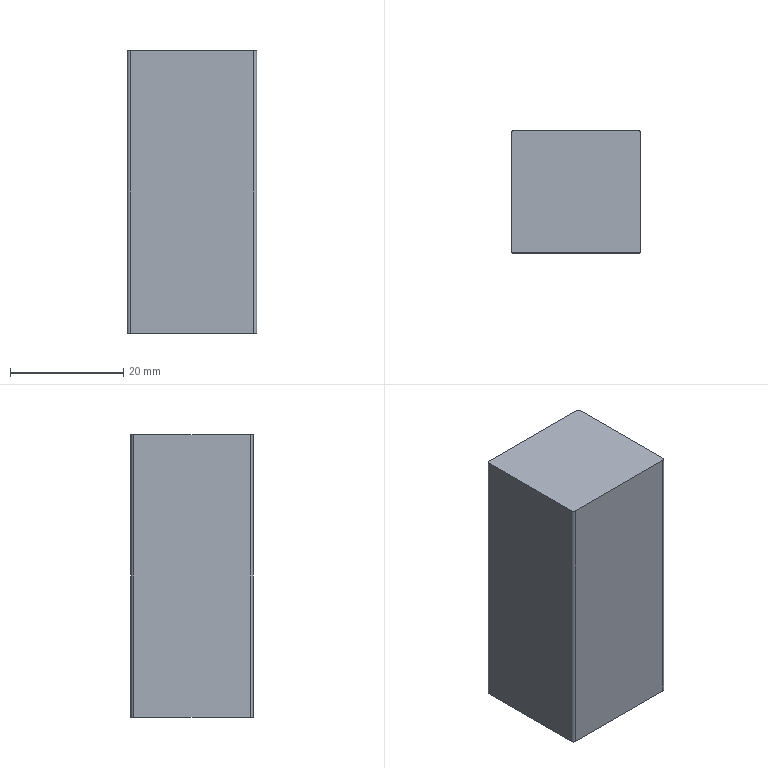Part | NX | features BREP 1 | 1 solid | 10 faces | box 22.899 x 21.607 x 50 mm | volume 24729 mm3 | plane 6 | cylinder 4 | commonest cylinder face diameters 1 x4
STEP:
#1=CARTESIAN_POINT('',(-10.95,10.804,-40.6));
#2=VERTEX_POINT('',#1);
#3=CARTESIAN_POINT('',(-11.45,10.304,-40.6));
#4=VERTEX_POINT('',#3);
#5=CARTESIAN_POINT('',(-10.95,10.304,-40.6));
#6=DIRECTION('',(0.,0.,1.));
#7=DIRECTION('',(1.,0.,0.));
#8=AXIS2_PLACEMENT_3D('',#5,#6,#7);
#9=CIRCLE('',#8,0.5);
#10=EDGE_CURVE('',#2,#4,#9,.T.);
#11=ORIENTED_EDGE('',*,*,#10,.F.);
#12=CARTESIAN_POINT('',(-10.95,10.804,-90.6));
#13=VERTEX_POINT('',#12);
#14=CARTESIAN_POINT('',(-10.95,10.804,-90.6));
#15=DIRECTION('',(0.,0.,1.));
#16=VECTOR('',#15,1000.);
#17=LINE('',#14,#16);
#18=EDGE_CURVE('',#13,#2,#17,.T.);
#19=ORIENTED_EDGE('',*,*,#18,.F.);
#20=CARTESIAN_POINT('',(-11.45,10.304,-90.6));
#21=VERTEX_POINT('',#20);
#22=CARTESIAN_POINT('',(-10.95,10.304,-90.6));
#23=DIRECTION('',(0.,0.,1.));
#24=DIRECTION('',(1.,0.,0.));
#25=AXIS2_PLACEMENT_3D('',#22,#23,#24);
#26=CIRCLE('',#25,0.5);
#27=EDGE_CURVE('',#13,#21,#26,.T.);
#28=ORIENTED_EDGE('',*,*,#27,.T.);
#29=CARTESIAN_POINT('',(-11.45,10.304,-90.6));
#30=DIRECTION('',(0.,0.,1.));
#31=VECTOR('',#30,1000.);
#32=LINE('',#29,#31);
#33=EDGE_CURVE('',#21,#4,#32,.T.);
#34=ORIENTED_EDGE('',*,*,#33,.T.);
#35=EDGE_LOOP('',(#11,#19,#28,#34));
#36=FACE_BOUND('',#35,.T.);
#37=CARTESIAN_POINT('',(-10.95,10.304,-90.6));
#38=DIRECTION('',(0.,0.,1.));
#39=DIRECTION('',(-1.,0.,0.));
#40=AXIS2_PLACEMENT_3D('',#37,#38,#39);
#41=CYLINDRICAL_SURFACE('',#40,0.5);
#42=ADVANCED_FACE('',(#36),#41,.T.);
#43=CARTESIAN_POINT('',(-11.45,-10.304,-40.6));
#44=VERTEX_POINT('',#43);
#45=CARTESIAN_POINT('',(-11.45,-10.304,-40.6));
#46=DIRECTION('',(0.,1.,0.));
#47=VECTOR('',#46,1000.);
#48=LINE('',#45,#47);
#49=EDGE_CURVE('',#44,#4,#48,.T.);
#50=ORIENTED_EDGE('',*,*,#49,.T.);
#51=ORIENTED_EDGE('',*,*,#33,.F.);
#52=CARTESIAN_POINT('',(-11.45,-10.304,-90.6));
#53=VERTEX_POINT('',#52);
#54=CARTESIAN_POINT('',(-11.45,-10.304,-90.6));
#55=DIRECTION('',(0.,1.,0.));
#56=VECTOR('',#55,1000.);
#57=LINE('',#54,#56);
#58=EDGE_CURVE('',#53,#21,#57,.T.);
#59=ORIENTED_EDGE('',*,*,#58,.F.);
#60=CARTESIAN_POINT('',(-11.45,-10.304,-90.6));
#61=DIRECTION('',(0.,0.,1.));
#62=VECTOR('',#61,1000.);
#63=LINE('',#60,#62);
#64=EDGE_CURVE('',#53,#44,#63,.T.);
#65=ORIENTED_EDGE('',*,*,#64,.T.);
#66=EDGE_LOOP('',(#50,#51,#59,#65));
#67=FACE_BOUND('',#66,.T.);
#68=CARTESIAN_POINT('',(-11.45,-10.304,-90.6));
#69=DIRECTION('',(1.,0.,0.));
#70=DIRECTION('',(0.,0.,1.));
#71=AXIS2_PLACEMENT_3D('',#68,#69,#70);
#72=PLANE('',#71);
#73=ADVANCED_FACE('',(#67),#72,.F.);
#74=CARTESIAN_POINT('',(-10.95,-10.804,-40.6));
#75=VERTEX_POINT('',#74);
#76=CARTESIAN_POINT('',(-10.95,-10.304,-40.6));
#77=DIRECTION('',(0.,0.,1.));
#78=DIRECTION('',(1.,0.,0.));
#79=AXIS2_PLACEMENT_3D('',#76,#77,#78);
#80=CIRCLE('',#79,0.5);
#81=EDGE_CURVE('',#44,#75,#80,.T.);
#82=ORIENTED_EDGE('',*,*,#81,.F.);
#83=ORIENTED_EDGE('',*,*,#64,.F.);
#84=CARTESIAN_POINT('',(-10.95,-10.804,-90.6));
#85=VERTEX_POINT('',#84);
#86=CARTESIAN_POINT('',(-10.95,-10.304,-90.6));
#87=DIRECTION('',(0.,0.,1.));
#88=DIRECTION('',(1.,0.,0.));
#89=AXIS2_PLACEMENT_3D('',#86,#87,#88);
#90=CIRCLE('',#89,0.5);
#91=EDGE_CURVE('',#53,#85,#90,.T.);
#92=ORIENTED_EDGE('',*,*,#91,.T.);
#93=CARTESIAN_POINT('',(-10.95,-10.804,-90.6));
#94=DIRECTION('',(0.,0.,1.));
#95=VECTOR('',#94,1000.);
#96=LINE('',#93,#95);
#97=EDGE_CURVE('',#85,#75,#96,.T.);
#98=ORIENTED_EDGE('',*,*,#97,.T.);
#99=EDGE_LOOP('',(#82,#83,#92,#98));
#100=FACE_BOUND('',#99,.T.);
#101=CARTESIAN_POINT('',(-10.95,-10.304,-90.6));
#102=DIRECTION('',(0.,0.,1.));
#103=DIRECTION('',(-1.,0.,0.));
#104=AXIS2_PLACEMENT_3D('',#101,#102,#103);
#105=CYLINDRICAL_SURFACE('',#104,0.5);
#106=ADVANCED_FACE('',(#100),#105,.T.);
#107=CARTESIAN_POINT('',(10.95,-10.804,-40.6));
#108=VERTEX_POINT('',#107);
#109=CARTESIAN_POINT('',(10.95,-10.804,-40.6));
#110=DIRECTION('',(-1.,0.,0.));
#111=VECTOR('',#110,1000.);
#112=LINE('',#109,#111);
#113=EDGE_CURVE('',#108,#75,#112,.T.);
#114=ORIENTED_EDGE('',*,*,#113,.T.);
#115=ORIENTED_EDGE('',*,*,#97,.F.);
#116=CARTESIAN_POINT('',(10.95,-10.804,-90.6));
#117=VERTEX_POINT('',#116);
#118=CARTESIAN_POINT('',(10.95,-10.804,-90.6));
#119=DIRECTION('',(-1.,0.,0.));
#120=VECTOR('',#119,1000.);
#121=LINE('',#118,#120);
#122=EDGE_CURVE('',#117,#85,#121,.T.);
#123=ORIENTED_EDGE('',*,*,#122,.F.);
#124=CARTESIAN_POINT('',(10.95,-10.804,-90.6));
#125=DIRECTION('',(0.,0.,1.));
#126=VECTOR('',#125,1000.);
#127=LINE('',#124,#126);
#128=EDGE_CURVE('',#117,#108,#127,.T.);
#129=ORIENTED_EDGE('',*,*,#128,.T.);
#130=EDGE_LOOP('',(#114,#115,#123,#129));
#131=FACE_BOUND('',#130,.T.);
#132=CARTESIAN_POINT('',(10.95,-10.804,-90.6));
#133=DIRECTION('',(0.,1.,0.));
#134=DIRECTION('',(0.,0.,-1.));
#135=AXIS2_PLACEMENT_3D('',#132,#133,#134);
#136=PLANE('',#135);
#137=ADVANCED_FACE('',(#131),#136,.F.);
#138=CARTESIAN_POINT('',(11.45,-10.304,-40.6));
#139=VERTEX_POINT('',#138);
#140=CARTESIAN_POINT('',(10.95,-10.304,-40.6));
#141=DIRECTION('',(0.,0.,1.));
#142=DIRECTION('',(1.,0.,0.));
#143=AXIS2_PLACEMENT_3D('',#140,#141,#142);
#144=CIRCLE('',#143,0.5);
#145=EDGE_CURVE('',#108,#139,#144,.T.);
#146=ORIENTED_EDGE('',*,*,#145,.F.);
#147=ORIENTED_EDGE('',*,*,#128,.F.);
#148=CARTESIAN_POINT('',(11.45,-10.304,-90.6));
#149=VERTEX_POINT('',#148);
#150=CARTESIAN_POINT('',(10.95,-10.304,-90.6));
#151=DIRECTION('',(0.,0.,1.));
#152=DIRECTION('',(1.,0.,0.));
#153=AXIS2_PLACEMENT_3D('',#150,#151,#152);
#154=CIRCLE('',#153,0.5);
#155=EDGE_CURVE('',#117,#149,#154,.T.);
#156=ORIENTED_EDGE('',*,*,#155,.T.);
#157=CARTESIAN_POINT('',(11.45,-10.304,-90.6));
#158=DIRECTION('',(0.,0.,1.));
#159=VECTOR('',#158,1000.);
#160=LINE('',#157,#159);
#161=EDGE_CURVE('',#149,#139,#160,.T.);
#162=ORIENTED_EDGE('',*,*,#161,.T.);
#163=EDGE_LOOP('',(#146,#147,#156,#162));
#164=FACE_BOUND('',#163,.T.);
#165=CARTESIAN_POINT('',(10.95,-10.304,-90.6));
#166=DIRECTION('',(0.,0.,1.));
#167=DIRECTION('',(-1.,0.,0.));
#168=AXIS2_PLACEMENT_3D('',#165,#166,#167);
#169=CYLINDRICAL_SURFACE('',#168,0.5);
#170=ADVANCED_FACE('',(#164),#169,.T.);
#171=CARTESIAN_POINT('',(11.45,10.304,-40.6));
#172=VERTEX_POINT('',#171);
#173=CARTESIAN_POINT('',(11.45,10.304,-40.6));
#174=DIRECTION('',(0.,-1.,0.));
#175=VECTOR('',#174,1000.);
#176=LINE('',#173,#175);
#177=EDGE_CURVE('',#172,#139,#176,.T.);
#178=ORIENTED_EDGE('',*,*,#177,.T.);
#179=ORIENTED_EDGE('',*,*,#161,.F.);
#180=CARTESIAN_POINT('',(11.45,10.304,-90.6));
#181=VERTEX_POINT('',#180);
#182=CARTESIAN_POINT('',(11.45,10.304,-90.6));
#183=DIRECTION('',(0.,-1.,0.));
#184=VECTOR('',#183,1000.);
#185=LINE('',#182,#184);
#186=EDGE_CURVE('',#181,#149,#185,.T.);
#187=ORIENTED_EDGE('',*,*,#186,.F.);
#188=CARTESIAN_POINT('',(11.45,10.304,-90.6));
#189=DIRECTION('',(0.,0.,1.));
#190=VECTOR('',#189,1000.);
#191=LINE('',#188,#190);
#192=EDGE_CURVE('',#181,#172,#191,.T.);
#193=ORIENTED_EDGE('',*,*,#192,.T.);
#194=EDGE_LOOP('',(#178,#179,#187,#193));
#195=FACE_BOUND('',#194,.T.);
#196=CARTESIAN_POINT('',(11.45,10.304,-90.6));
#197=DIRECTION('',(-1.,0.,0.));
#198=DIRECTION('',(0.,1.,0.));
#199=AXIS2_PLACEMENT_3D('',#196,#197,#198);
#200=PLANE('',#199);
#201=ADVANCED_FACE('',(#195),#200,.F.);
#202=CARTESIAN_POINT('',(10.95,10.804,-40.6));
#203=VERTEX_POINT('',#202);
#204=CARTESIAN_POINT('',(10.95,10.304,-40.6));
#205=DIRECTION('',(0.,0.,1.));
#206=DIRECTION('',(1.,0.,0.));
#207=AXIS2_PLACEMENT_3D('',#204,#205,#206);
#208=CIRCLE('',#207,0.5);
#209=EDGE_CURVE('',#172,#203,#208,.T.);
#210=ORIENTED_EDGE('',*,*,#209,.F.);
#211=ORIENTED_EDGE('',*,*,#192,.F.);
#212=CARTESIAN_POINT('',(10.95,10.804,-90.6));
#213=VERTEX_POINT('',#212);
#214=CARTESIAN_POINT('',(10.95,10.304,-90.6));
#215=DIRECTION('',(0.,0.,1.));
#216=DIRECTION('',(1.,0.,0.));
#217=AXIS2_PLACEMENT_3D('',#214,#215,#216);
#218=CIRCLE('',#217,0.5);
#219=EDGE_CURVE('',#181,#213,#218,.T.);
#220=ORIENTED_EDGE('',*,*,#219,.T.);
#221=CARTESIAN_POINT('',(10.95,10.804,-90.6));
#222=DIRECTION('',(0.,0.,1.));
#223=VECTOR('',#222,1000.);
#224=LINE('',#221,#223);
#225=EDGE_CURVE('',#213,#203,#224,.T.);
#226=ORIENTED_EDGE('',*,*,#225,.T.);
#227=EDGE_LOOP('',(#210,#211,#220,#226));
#228=FACE_BOUND('',#227,.T.);
#229=CARTESIAN_POINT('',(10.95,10.304,-90.6));
#230=DIRECTION('',(0.,0.,1.));
#231=DIRECTION('',(-1.,0.,0.));
#232=AXIS2_PLACEMENT_3D('',#229,#230,#231);
#233=CYLINDRICAL_SURFACE('',#232,0.5);
#234=ADVANCED_FACE('',(#228),#233,.T.);
#235=CARTESIAN_POINT('',(-10.95,10.804,-40.6));
#236=DIRECTION('',(1.,0.,0.));
#237=VECTOR('',#236,1000.);
#238=LINE('',#235,#237);
#239=EDGE_CURVE('',#2,#203,#238,.T.);
#240=ORIENTED_EDGE('',*,*,#239,.T.);
#241=ORIENTED_EDGE('',*,*,#225,.F.);
#242=CARTESIAN_POINT('',(-10.95,10.804,-90.6));
#243=DIRECTION('',(1.,0.,0.));
#244=VECTOR('',#243,1000.);
#245=LINE('',#242,#244);
#246=EDGE_CURVE('',#13,#213,#245,.T.);
#247=ORIENTED_EDGE('',*,*,#246,.F.);
#248=ORIENTED_EDGE('',*,*,#18,.T.);
#249=EDGE_LOOP('',(#240,#241,#247,#248));
#250=FACE_BOUND('',#249,.T.);
#251=CARTESIAN_POINT('',(-10.95,10.804,-90.6));
#252=DIRECTION('',(0.,-1.,0.));
#253=DIRECTION('',(-1.,0.,0.));
#254=AXIS2_PLACEMENT_3D('',#251,#252,#253);
#255=PLANE('',#254);
#256=ADVANCED_FACE('',(#250),#255,.F.);
#257=ORIENTED_EDGE('',*,*,#27,.F.);
#258=ORIENTED_EDGE('',*,*,#246,.T.);
#259=ORIENTED_EDGE('',*,*,#219,.F.);
#260=ORIENTED_EDGE('',*,*,#186,.T.);
#261=ORIENTED_EDGE('',*,*,#155,.F.);
#262=ORIENTED_EDGE('',*,*,#122,.T.);
#263=ORIENTED_EDGE('',*,*,#91,.F.);
#264=ORIENTED_EDGE('',*,*,#58,.T.);
#265=EDGE_LOOP('',(#257,#258,#259,#260,#261,#262,#263,#264));
#266=FACE_BOUND('',#265,.T.);
#267=CARTESIAN_POINT('',(-10.95,10.304,-90.6));
#268=DIRECTION('',(0.,0.,1.));
#269=DIRECTION('',(-1.,0.,0.));
#270=AXIS2_PLACEMENT_3D('',#267,#268,#269);
#271=PLANE('',#270);
#272=ADVANCED_FACE('',(#266),#271,.F.);
#273=ORIENTED_EDGE('',*,*,#10,.T.);
#274=ORIENTED_EDGE('',*,*,#49,.F.);
#275=ORIENTED_EDGE('',*,*,#81,.T.);
#276=ORIENTED_EDGE('',*,*,#113,.F.);
#277=ORIENTED_EDGE('',*,*,#145,.T.);
#278=ORIENTED_EDGE('',*,*,#177,.F.);
#279=ORIENTED_EDGE('',*,*,#209,.T.);
#280=ORIENTED_EDGE('',*,*,#239,.F.);
#281=EDGE_LOOP('',(#273,#274,#275,#276,#277,#278,#279,#280));
#282=FACE_BOUND('',#281,.T.);
#283=CARTESIAN_POINT('',(-10.95,10.304,-40.6));
#284=DIRECTION('',(0.,0.,1.));
#285=DIRECTION('',(-1.,0.,0.));
#286=AXIS2_PLACEMENT_3D('',#283,#284,#285);
#287=PLANE('',#286);
#288=ADVANCED_FACE('',(#282),#287,.T.);
#289=CLOSED_SHELL('',(#42,#73,#106,#137,#170,#201,#234,#256,#272,#288));
#290=MANIFOLD_SOLID_BREP('',#289);
#291=(LENGTH_UNIT()NAMED_UNIT(*)SI_UNIT(.MILLI.,.METRE.));
#292=UNCERTAINTY_MEASURE_WITH_UNIT(LENGTH_MEASURE(0.00001),#291,'','');
#293=(NAMED_UNIT(*)PLANE_ANGLE_UNIT()SI_UNIT($,.RADIAN.));
#294=(NAMED_UNIT(*)SI_UNIT($,.STERADIAN.)SOLID_ANGLE_UNIT());
#295=(GEOMETRIC_REPRESENTATION_CONTEXT(3)GLOBAL_UNCERTAINTY_ASSIGNED_CONTEXT((#292))GLOBAL_UNIT_ASSIGNED_CONTEXT((#291,#293,#294))REPRESENTATION_CONTEXT('',''));
#296=ADVANCED_BREP_SHAPE_REPRESENTATION('',(#290),#295);